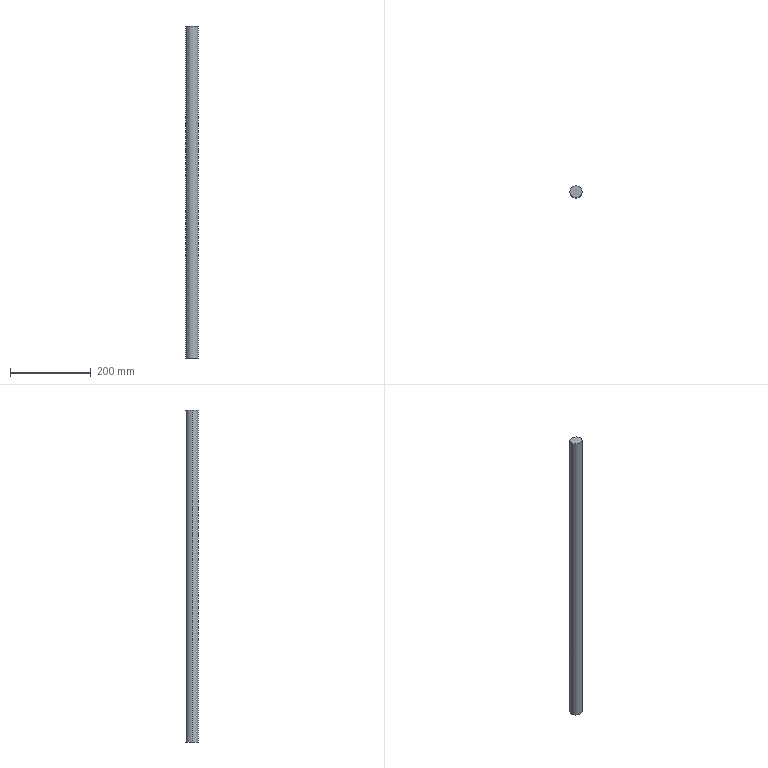Part | SolidWorks | features BaseBody 1 | 1 solid | 8 faces | box 30 x 30 x 820 mm | volume 578882 mm3 | cylinder 4 | cone 2 | plane 2 | commonest cylinder face diameters 6.8 x2 30 x2
STEP:
#1=CARTESIAN_POINT('',(3.4,0.,-390.25));
#2=VERTEX_POINT('',#1);
#3=CARTESIAN_POINT('',(3.4,0.,-410.));
#4=VERTEX_POINT('',#3);
#5=CARTESIAN_POINT('',(3.4,0.,-410.));
#6=DIRECTION('',(0.,0.,-1.));
#7=VECTOR('',#6,1000.);
#8=LINE('',#5,#7);
#9=EDGE_CURVE('',#2,#4,#8,.T.);
#10=ORIENTED_EDGE('',*,*,#9,.F.);
#11=CARTESIAN_POINT('',(-3.4,0.,-390.25));
#12=VERTEX_POINT('',#11);
#13=CARTESIAN_POINT('',(0.,0.,-390.25));
#14=DIRECTION('',(0.,0.,-1.));
#15=DIRECTION('',(-1.,0.,0.));
#16=AXIS2_PLACEMENT_3D('',#13,#14,#15);
#17=CIRCLE('',#16,3.4);
#18=EDGE_CURVE('',#12,#2,#17,.T.);
#19=ORIENTED_EDGE('',*,*,#18,.F.);
#20=CARTESIAN_POINT('',(-3.4,0.,-410.));
#21=VERTEX_POINT('',#20);
#22=CARTESIAN_POINT('',(-3.4,0.,-410.));
#23=DIRECTION('',(0.,0.,-1.));
#24=VECTOR('',#23,1000.);
#25=LINE('',#22,#24);
#26=EDGE_CURVE('',#12,#21,#25,.T.);
#27=ORIENTED_EDGE('',*,*,#26,.T.);
#28=CARTESIAN_POINT('',(0.,0.,-410.));
#29=DIRECTION('',(0.,0.,-1.));
#30=DIRECTION('',(-1.,0.,0.));
#31=AXIS2_PLACEMENT_3D('',#28,#29,#30);
#32=CIRCLE('',#31,3.4);
#33=EDGE_CURVE('',#21,#4,#32,.T.);
#34=ORIENTED_EDGE('',*,*,#33,.T.);
#35=EDGE_LOOP('',(#10,#19,#27,#34));
#36=FACE_OUTER_BOUND('',#35,.T.);
#37=CARTESIAN_POINT('',(0.,0.,-410.));
#38=DIRECTION('',(0.,0.,-1.));
#39=DIRECTION('',(-1.,0.,0.));
#40=AXIS2_PLACEMENT_3D('',#37,#38,#39);
#41=CYLINDRICAL_SURFACE('',#40,3.4);
#42=ADVANCED_FACE('',(#36),#41,.F.);
#43=CARTESIAN_POINT('',(0.,0.,-388.207));
#44=VERTEX_POINT('',#43);
#45=CARTESIAN_POINT('',(3.4,0.,-390.25));
#46=DIRECTION('',(0.8572,0.,-0.515));
#47=VECTOR('',#46,1000.);
#48=LINE('',#45,#47);
#49=EDGE_CURVE('',#44,#2,#48,.T.);
#50=ORIENTED_EDGE('',*,*,#49,.F.);
#51=CARTESIAN_POINT('',(-3.4,0.,-390.25));
#52=DIRECTION('',(-0.8572,0.,-0.515));
#53=VECTOR('',#52,1000.);
#54=LINE('',#51,#53);
#55=EDGE_CURVE('',#44,#12,#54,.T.);
#56=ORIENTED_EDGE('',*,*,#55,.T.);
#57=ORIENTED_EDGE('',*,*,#18,.T.);
#58=EDGE_LOOP('',(#50,#56,#57));
#59=FACE_OUTER_BOUND('',#58,.T.);
#60=CARTESIAN_POINT('',(0.,0.,-390.25));
#61=DIRECTION('',(0.,0.,-1.));
#62=DIRECTION('',(-1.,0.,0.));
#63=AXIS2_PLACEMENT_3D('',#60,#61,#62);
#64=CONICAL_SURFACE('',#63,3.4,1.03);
#65=ADVANCED_FACE('',(#59),#64,.F.);
#66=ORIENTED_EDGE('',*,*,#33,.F.);
#67=CARTESIAN_POINT('',(0.,0.,-410.));
#68=DIRECTION('',(0.,0.,-1.));
#69=DIRECTION('',(-1.,0.,0.));
#70=AXIS2_PLACEMENT_3D('',#67,#68,#69);
#71=CIRCLE('',#70,3.4);
#72=EDGE_CURVE('',#4,#21,#71,.T.);
#73=ORIENTED_EDGE('',*,*,#72,.F.);
#74=EDGE_LOOP('',(#66,#73));
#75=FACE_BOUND('',#74,.T.);
#76=CARTESIAN_POINT('',(-15.,0.,-410.));
#77=VERTEX_POINT('',#76);
#78=CARTESIAN_POINT('',(15.,0.,-410.));
#79=VERTEX_POINT('',#78);
#80=CARTESIAN_POINT('',(0.,0.,-410.));
#81=DIRECTION('',(0.,0.,1.));
#82=DIRECTION('',(1.,0.,0.));
#83=AXIS2_PLACEMENT_3D('',#80,#81,#82);
#84=CIRCLE('',#83,15.);
#85=EDGE_CURVE('',#77,#79,#84,.T.);
#86=ORIENTED_EDGE('',*,*,#85,.F.);
#87=CARTESIAN_POINT('',(0.,0.,-410.));
#88=DIRECTION('',(0.,0.,1.));
#89=DIRECTION('',(1.,0.,0.));
#90=AXIS2_PLACEMENT_3D('',#87,#88,#89);
#91=CIRCLE('',#90,15.);
#92=EDGE_CURVE('',#79,#77,#91,.T.);
#93=ORIENTED_EDGE('',*,*,#92,.F.);
#94=EDGE_LOOP('',(#86,#93));
#95=FACE_OUTER_BOUND('',#94,.T.);
#96=CARTESIAN_POINT('',(0.,0.,-410.));
#97=DIRECTION('',(0.,0.,1.));
#98=DIRECTION('',(1.,0.,0.));
#99=AXIS2_PLACEMENT_3D('',#96,#97,#98);
#100=PLANE('',#99);
#101=ADVANCED_FACE('',(#75,#95),#100,.F.);
#102=CARTESIAN_POINT('',(-15.,0.,410.));
#103=VERTEX_POINT('',#102);
#104=CARTESIAN_POINT('',(15.,0.,410.));
#105=VERTEX_POINT('',#104);
#106=CARTESIAN_POINT('',(0.,0.,410.));
#107=DIRECTION('',(0.,0.,1.));
#108=DIRECTION('',(1.,0.,0.));
#109=AXIS2_PLACEMENT_3D('',#106,#107,#108);
#110=CIRCLE('',#109,15.);
#111=EDGE_CURVE('',#103,#105,#110,.T.);
#112=ORIENTED_EDGE('',*,*,#111,.T.);
#113=CARTESIAN_POINT('',(0.,0.,410.));
#114=DIRECTION('',(0.,0.,1.));
#115=DIRECTION('',(1.,0.,0.));
#116=AXIS2_PLACEMENT_3D('',#113,#114,#115);
#117=CIRCLE('',#116,15.);
#118=EDGE_CURVE('',#105,#103,#117,.T.);
#119=ORIENTED_EDGE('',*,*,#118,.T.);
#120=EDGE_LOOP('',(#112,#119));
#121=FACE_OUTER_BOUND('',#120,.T.);
#122=CARTESIAN_POINT('',(0.,0.,410.));
#123=DIRECTION('',(0.,0.,1.));
#124=DIRECTION('',(1.,0.,0.));
#125=AXIS2_PLACEMENT_3D('',#122,#123,#124);
#126=PLANE('',#125);
#127=ADVANCED_FACE('',(#121),#126,.T.);
#128=CARTESIAN_POINT('',(15.,0.,410.));
#129=DIRECTION('',(0.,0.,-1.));
#130=VECTOR('',#129,1000.);
#131=LINE('',#128,#130);
#132=EDGE_CURVE('',#105,#79,#131,.T.);
#133=ORIENTED_EDGE('',*,*,#132,.F.);
#134=ORIENTED_EDGE('',*,*,#111,.F.);
#135=CARTESIAN_POINT('',(-15.,0.,410.));
#136=DIRECTION('',(0.,0.,-1.));
#137=VECTOR('',#136,1000.);
#138=LINE('',#135,#137);
#139=EDGE_CURVE('',#103,#77,#138,.T.);
#140=ORIENTED_EDGE('',*,*,#139,.T.);
#141=ORIENTED_EDGE('',*,*,#85,.T.);
#142=EDGE_LOOP('',(#133,#134,#140,#141));
#143=FACE_OUTER_BOUND('',#142,.T.);
#144=CARTESIAN_POINT('',(0.,0.,410.));
#145=DIRECTION('',(0.,0.,-1.));
#146=DIRECTION('',(-1.,0.,0.));
#147=AXIS2_PLACEMENT_3D('',#144,#145,#146);
#148=CYLINDRICAL_SURFACE('',#147,15.);
#149=ADVANCED_FACE('',(#143),#148,.T.);
#150=ORIENTED_EDGE('',*,*,#118,.F.);
#151=ORIENTED_EDGE('',*,*,#132,.T.);
#152=ORIENTED_EDGE('',*,*,#92,.T.);
#153=ORIENTED_EDGE('',*,*,#139,.F.);
#154=EDGE_LOOP('',(#150,#151,#152,#153));
#155=FACE_OUTER_BOUND('',#154,.T.);
#156=CARTESIAN_POINT('',(0.,0.,410.));
#157=DIRECTION('',(0.,0.,-1.));
#158=DIRECTION('',(-1.,0.,0.));
#159=AXIS2_PLACEMENT_3D('',#156,#157,#158);
#160=CYLINDRICAL_SURFACE('',#159,15.);
#161=ADVANCED_FACE('',(#155),#160,.T.);
#162=ORIENTED_EDGE('',*,*,#55,.F.);
#163=ORIENTED_EDGE('',*,*,#49,.T.);
#164=CARTESIAN_POINT('',(0.,0.,-390.25));
#165=DIRECTION('',(0.,0.,-1.));
#166=DIRECTION('',(-1.,0.,0.));
#167=AXIS2_PLACEMENT_3D('',#164,#165,#166);
#168=CIRCLE('',#167,3.4);
#169=EDGE_CURVE('',#2,#12,#168,.T.);
#170=ORIENTED_EDGE('',*,*,#169,.T.);
#171=EDGE_LOOP('',(#162,#163,#170));
#172=FACE_OUTER_BOUND('',#171,.T.);
#173=CARTESIAN_POINT('',(0.,0.,-390.25));
#174=DIRECTION('',(0.,0.,-1.));
#175=DIRECTION('',(-1.,0.,0.));
#176=AXIS2_PLACEMENT_3D('',#173,#174,#175);
#177=CONICAL_SURFACE('',#176,3.4,1.03);
#178=ADVANCED_FACE('',(#172),#177,.F.);
#179=ORIENTED_EDGE('',*,*,#169,.F.);
#180=ORIENTED_EDGE('',*,*,#9,.T.);
#181=ORIENTED_EDGE('',*,*,#72,.T.);
#182=ORIENTED_EDGE('',*,*,#26,.F.);
#183=EDGE_LOOP('',(#179,#180,#181,#182));
#184=FACE_OUTER_BOUND('',#183,.T.);
#185=CARTESIAN_POINT('',(0.,0.,-410.));
#186=DIRECTION('',(0.,0.,-1.));
#187=DIRECTION('',(-1.,0.,0.));
#188=AXIS2_PLACEMENT_3D('',#185,#186,#187);
#189=CYLINDRICAL_SURFACE('',#188,3.4);
#190=ADVANCED_FACE('',(#184),#189,.F.);
#191=CLOSED_SHELL('',(#42,#65,#101,#127,#149,#161,#178,#190));
#192=MANIFOLD_SOLID_BREP('',#191);
#193=CARTESIAN_POINT('',(0.,0.,0.));
#194=DIRECTION('',(0.,0.,1.));
#195=DIRECTION('',(1.,0.,0.));
#196=AXIS2_PLACEMENT_3D('',#193,#194,#195);
#197=(LENGTH_UNIT()NAMED_UNIT(*)SI_UNIT(.MILLI.,.METRE.));
#198=UNCERTAINTY_MEASURE_WITH_UNIT(LENGTH_MEASURE(0.00001),#197,'','');
#199=(NAMED_UNIT(*)PLANE_ANGLE_UNIT()SI_UNIT($,.RADIAN.));
#200=(NAMED_UNIT(*)SI_UNIT($,.STERADIAN.)SOLID_ANGLE_UNIT());
#201=(GEOMETRIC_REPRESENTATION_CONTEXT(3)GLOBAL_UNCERTAINTY_ASSIGNED_CONTEXT((#198))GLOBAL_UNIT_ASSIGNED_CONTEXT((#197,#199,#200))REPRESENTATION_CONTEXT('',''));
#202=ADVANCED_BREP_SHAPE_REPRESENTATION('',(#192,#196),#201);